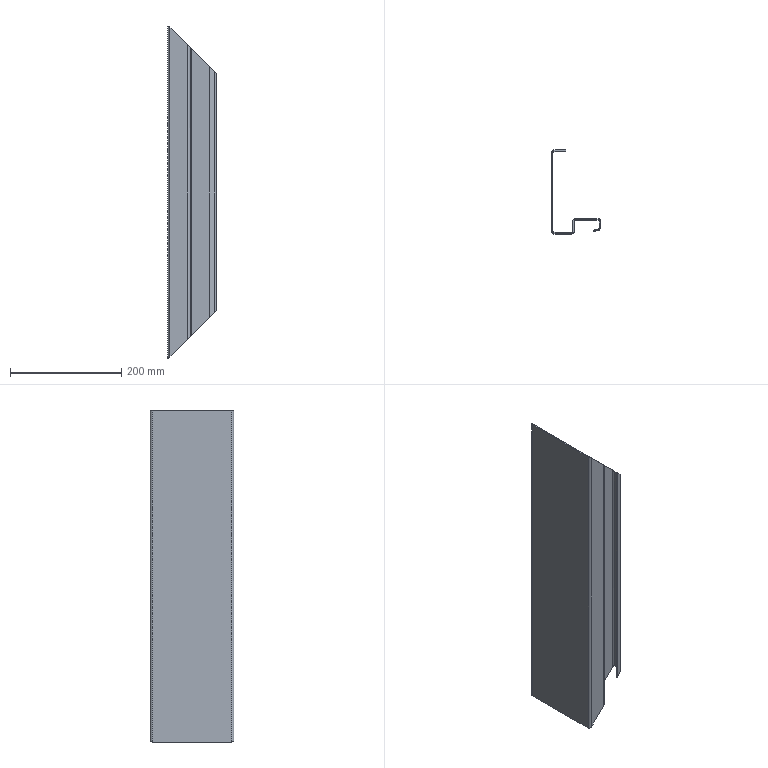Part | STEP file | 750038404 | 1 solid | 54 faces | box 87 x 150 x 596 mm | volume 335193 mm3 | plane 30 | cylinder 12 | spline 12 | commonest cylinder face diameters 4 x6 8 x6